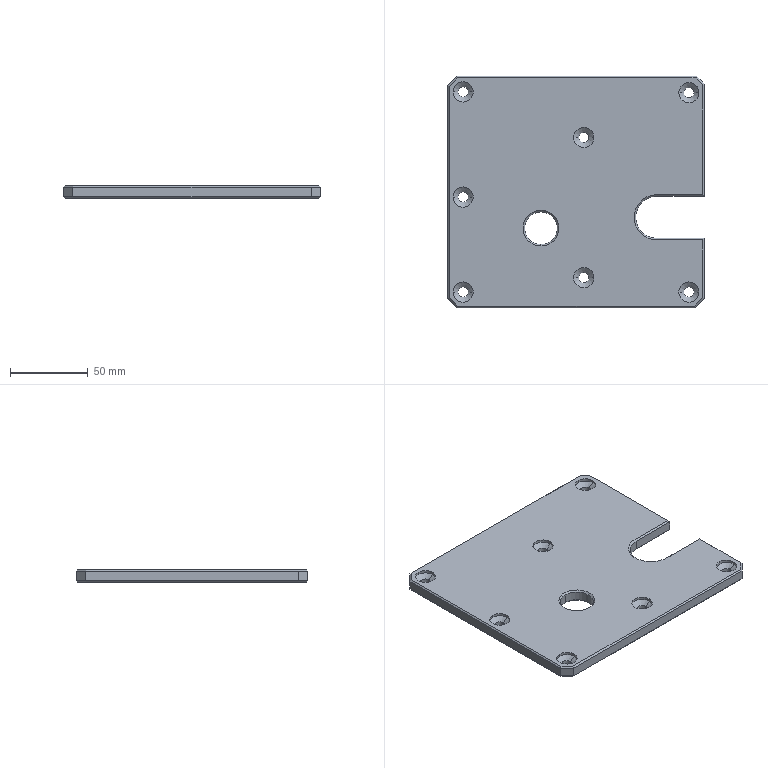Part | Creo | 1 solid | 88 faces | box 165 x 148.5 x 8 mm | volume 179149 mm3 | plane 37 | cylinder 31 | cone 20 | commonest cylinder face diameters 6.6 x14 13 x14 21 x2 27 x1